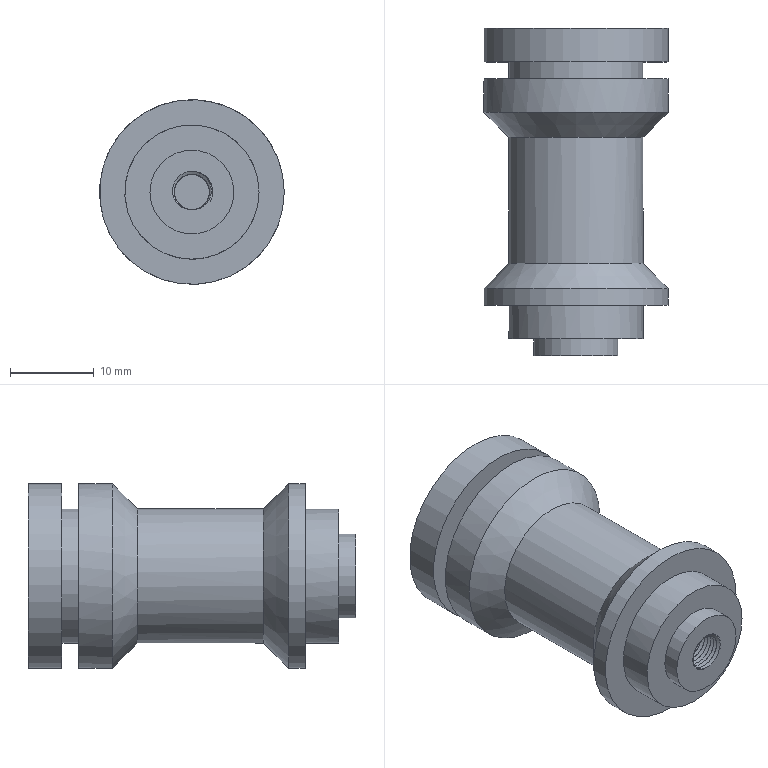Part | NX | features DATUM_CSYS 9, EXTRUDE 8, SKETCH 8, CHAMFER 2, THREADS 1 | 1 solid | 24 faces | box 22 x 39 x 22 mm | volume 9431 mm3 | cylinder 10 | plane 9 | spline 3 | cone 2 | commonest cylinder face diameters 16 x3 22 x3 4.2 x1 5 x1 6.5 x1 10 x1